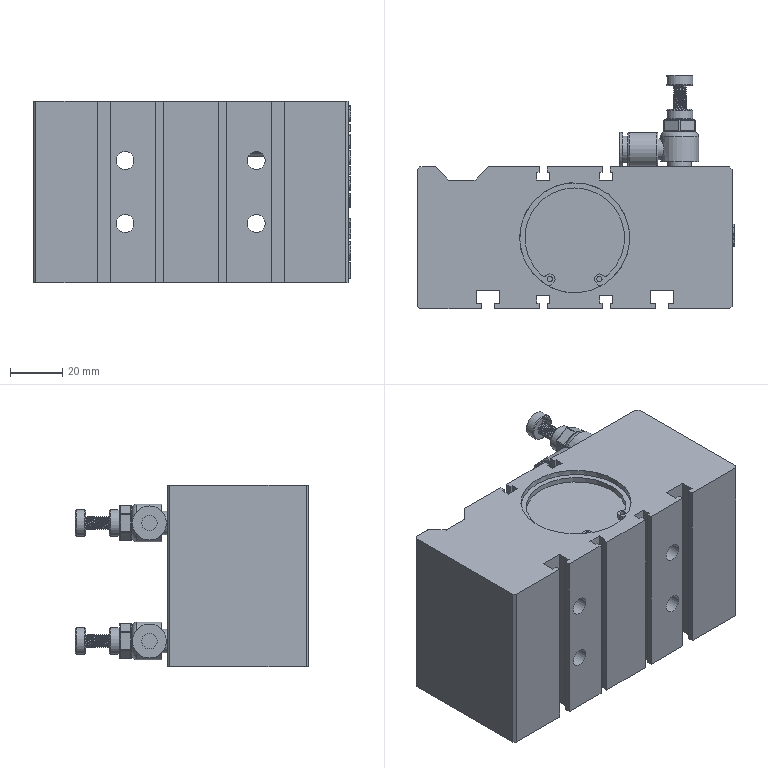Part | STEP file | Tube necking machine_id418_x_t | 1 solid | 353 faces | box 121 x 89 x 69 mm | volume 423791 mm3 | plane 237 | other 56 | cylinder 40 | cone 8 | spline 6 | torus 6 | commonest cylinder face diameters 10 x6 2 x4 6.8 x4 11 x4 13 x4 2.689 x2